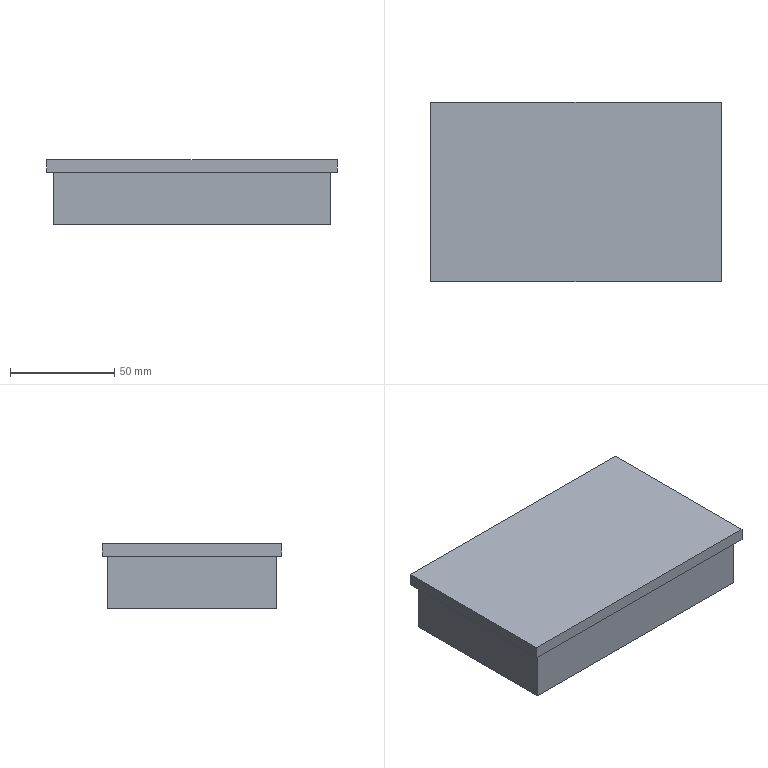Part | STEP file | Touch screen | 1 solid | 11 faces | box 139 x 86 x 31 mm | volume 341049 mm3 | plane 11
STEP:
#1=CARTESIAN_POINT('',(-66.5,40.5,0.));
#2=VERTEX_POINT('',#1);
#3=CARTESIAN_POINT('',(-66.5,-40.5,0.));
#4=VERTEX_POINT('',#3);
#5=CARTESIAN_POINT('',(-66.5,-40.5,0.));
#6=DIRECTION('',(0.,-1.,0.));
#7=VECTOR('',#6,1000.);
#8=LINE('',#5,#7);
#9=EDGE_CURVE('',#2,#4,#8,.T.);
#10=ORIENTED_EDGE('',*,*,#9,.T.);
#11=CARTESIAN_POINT('',(-66.5,-40.5,25.));
#12=VERTEX_POINT('',#11);
#13=CARTESIAN_POINT('',(-66.5,-40.5,25.));
#14=DIRECTION('',(0.,0.,-1.));
#15=VECTOR('',#14,1000.);
#16=LINE('',#13,#15);
#17=EDGE_CURVE('',#12,#4,#16,.T.);
#18=ORIENTED_EDGE('',*,*,#17,.F.);
#19=CARTESIAN_POINT('',(-66.5,40.5,25.));
#20=VERTEX_POINT('',#19);
#21=CARTESIAN_POINT('',(-66.5,-40.5,25.));
#22=DIRECTION('',(0.,-1.,0.));
#23=VECTOR('',#22,1000.);
#24=LINE('',#21,#23);
#25=EDGE_CURVE('',#20,#12,#24,.T.);
#26=ORIENTED_EDGE('',*,*,#25,.F.);
#27=CARTESIAN_POINT('',(-66.5,40.5,25.));
#28=DIRECTION('',(0.,0.,-1.));
#29=VECTOR('',#28,1000.);
#30=LINE('',#27,#29);
#31=EDGE_CURVE('',#20,#2,#30,.T.);
#32=ORIENTED_EDGE('',*,*,#31,.T.);
#33=EDGE_LOOP('',(#10,#18,#26,#32));
#34=FACE_OUTER_BOUND('',#33,.T.);
#35=CARTESIAN_POINT('',(-66.5,-40.5,25.));
#36=DIRECTION('',(1.,0.,0.));
#37=DIRECTION('',(0.,0.,-1.));
#38=AXIS2_PLACEMENT_3D('',#35,#36,#37);
#39=PLANE('',#38);
#40=ADVANCED_FACE('',(#34),#39,.F.);
#41=CARTESIAN_POINT('',(66.5,-40.5,0.));
#42=VERTEX_POINT('',#41);
#43=CARTESIAN_POINT('',(66.5,-40.5,0.));
#44=DIRECTION('',(1.,0.,0.));
#45=VECTOR('',#44,1000.);
#46=LINE('',#43,#45);
#47=EDGE_CURVE('',#4,#42,#46,.T.);
#48=ORIENTED_EDGE('',*,*,#47,.T.);
#49=CARTESIAN_POINT('',(66.5,-40.5,25.));
#50=VERTEX_POINT('',#49);
#51=CARTESIAN_POINT('',(66.5,-40.5,25.));
#52=DIRECTION('',(0.,0.,-1.));
#53=VECTOR('',#52,1000.);
#54=LINE('',#51,#53);
#55=EDGE_CURVE('',#50,#42,#54,.T.);
#56=ORIENTED_EDGE('',*,*,#55,.F.);
#57=CARTESIAN_POINT('',(66.5,-40.5,25.));
#58=DIRECTION('',(1.,0.,0.));
#59=VECTOR('',#58,1000.);
#60=LINE('',#57,#59);
#61=EDGE_CURVE('',#12,#50,#60,.T.);
#62=ORIENTED_EDGE('',*,*,#61,.F.);
#63=ORIENTED_EDGE('',*,*,#17,.T.);
#64=EDGE_LOOP('',(#48,#56,#62,#63));
#65=FACE_OUTER_BOUND('',#64,.T.);
#66=CARTESIAN_POINT('',(66.5,-40.5,25.));
#67=DIRECTION('',(0.,1.,0.));
#68=DIRECTION('',(0.,0.,1.));
#69=AXIS2_PLACEMENT_3D('',#66,#67,#68);
#70=PLANE('',#69);
#71=ADVANCED_FACE('',(#65),#70,.F.);
#72=CARTESIAN_POINT('',(66.5,40.5,0.));
#73=VERTEX_POINT('',#72);
#74=CARTESIAN_POINT('',(66.5,-40.5,0.));
#75=DIRECTION('',(0.,1.,0.));
#76=VECTOR('',#75,1000.);
#77=LINE('',#74,#76);
#78=EDGE_CURVE('',#42,#73,#77,.T.);
#79=ORIENTED_EDGE('',*,*,#78,.T.);
#80=CARTESIAN_POINT('',(66.5,40.5,25.));
#81=VERTEX_POINT('',#80);
#82=CARTESIAN_POINT('',(66.5,40.5,25.));
#83=DIRECTION('',(0.,0.,-1.));
#84=VECTOR('',#83,1000.);
#85=LINE('',#82,#84);
#86=EDGE_CURVE('',#81,#73,#85,.T.);
#87=ORIENTED_EDGE('',*,*,#86,.F.);
#88=CARTESIAN_POINT('',(66.5,-40.5,25.));
#89=DIRECTION('',(0.,1.,0.));
#90=VECTOR('',#89,1000.);
#91=LINE('',#88,#90);
#92=EDGE_CURVE('',#50,#81,#91,.T.);
#93=ORIENTED_EDGE('',*,*,#92,.F.);
#94=ORIENTED_EDGE('',*,*,#55,.T.);
#95=EDGE_LOOP('',(#79,#87,#93,#94));
#96=FACE_OUTER_BOUND('',#95,.T.);
#97=CARTESIAN_POINT('',(66.5,-40.5,25.));
#98=DIRECTION('',(-1.,0.,0.));
#99=DIRECTION('',(0.,0.,1.));
#100=AXIS2_PLACEMENT_3D('',#97,#98,#99);
#101=PLANE('',#100);
#102=ADVANCED_FACE('',(#96),#101,.F.);
#103=CARTESIAN_POINT('',(66.5,40.5,0.));
#104=DIRECTION('',(-1.,0.,0.));
#105=VECTOR('',#104,1000.);
#106=LINE('',#103,#105);
#107=EDGE_CURVE('',#73,#2,#106,.T.);
#108=ORIENTED_EDGE('',*,*,#107,.T.);
#109=ORIENTED_EDGE('',*,*,#31,.F.);
#110=CARTESIAN_POINT('',(66.5,40.5,25.));
#111=DIRECTION('',(-1.,0.,0.));
#112=VECTOR('',#111,1000.);
#113=LINE('',#110,#112);
#114=EDGE_CURVE('',#81,#20,#113,.T.);
#115=ORIENTED_EDGE('',*,*,#114,.F.);
#116=ORIENTED_EDGE('',*,*,#86,.T.);
#117=EDGE_LOOP('',(#108,#109,#115,#116));
#118=FACE_OUTER_BOUND('',#117,.T.);
#119=CARTESIAN_POINT('',(66.5,40.5,25.));
#120=DIRECTION('',(0.,-1.,0.));
#121=DIRECTION('',(0.,0.,-1.));
#122=AXIS2_PLACEMENT_3D('',#119,#120,#121);
#123=PLANE('',#122);
#124=ADVANCED_FACE('',(#118),#123,.F.);
#125=ORIENTED_EDGE('',*,*,#9,.F.);
#126=ORIENTED_EDGE('',*,*,#107,.F.);
#127=ORIENTED_EDGE('',*,*,#78,.F.);
#128=ORIENTED_EDGE('',*,*,#47,.F.);
#129=EDGE_LOOP('',(#125,#126,#127,#128));
#130=FACE_OUTER_BOUND('',#129,.T.);
#131=CARTESIAN_POINT('',(0.,0.,0.));
#132=DIRECTION('',(0.,0.,1.));
#133=DIRECTION('',(1.,0.,0.));
#134=AXIS2_PLACEMENT_3D('',#131,#132,#133);
#135=PLANE('',#134);
#136=ADVANCED_FACE('',(#130),#135,.F.);
#137=CARTESIAN_POINT('',(-69.5,43.,25.));
#138=VERTEX_POINT('',#137);
#139=CARTESIAN_POINT('',(-69.5,-43.,25.));
#140=VERTEX_POINT('',#139);
#141=CARTESIAN_POINT('',(-69.5,-43.,25.));
#142=DIRECTION('',(0.,-1.,0.));
#143=VECTOR('',#142,1000.);
#144=LINE('',#141,#143);
#145=EDGE_CURVE('',#138,#140,#144,.T.);
#146=ORIENTED_EDGE('',*,*,#145,.F.);
#147=CARTESIAN_POINT('',(69.5,43.,25.));
#148=VERTEX_POINT('',#147);
#149=CARTESIAN_POINT('',(69.5,43.,25.));
#150=DIRECTION('',(-1.,0.,0.));
#151=VECTOR('',#150,1000.);
#152=LINE('',#149,#151);
#153=EDGE_CURVE('',#148,#138,#152,.T.);
#154=ORIENTED_EDGE('',*,*,#153,.F.);
#155=CARTESIAN_POINT('',(69.5,-43.,25.));
#156=VERTEX_POINT('',#155);
#157=CARTESIAN_POINT('',(69.5,-43.,25.));
#158=DIRECTION('',(0.,1.,0.));
#159=VECTOR('',#158,1000.);
#160=LINE('',#157,#159);
#161=EDGE_CURVE('',#156,#148,#160,.T.);
#162=ORIENTED_EDGE('',*,*,#161,.F.);
#163=CARTESIAN_POINT('',(69.5,-43.,25.));
#164=DIRECTION('',(1.,0.,0.));
#165=VECTOR('',#164,1000.);
#166=LINE('',#163,#165);
#167=EDGE_CURVE('',#140,#156,#166,.T.);
#168=ORIENTED_EDGE('',*,*,#167,.F.);
#169=EDGE_LOOP('',(#146,#154,#162,#168));
#170=FACE_OUTER_BOUND('',#169,.T.);
#171=ORIENTED_EDGE('',*,*,#114,.T.);
#172=ORIENTED_EDGE('',*,*,#25,.T.);
#173=ORIENTED_EDGE('',*,*,#61,.T.);
#174=ORIENTED_EDGE('',*,*,#92,.T.);
#175=EDGE_LOOP('',(#171,#172,#173,#174));
#176=FACE_BOUND('',#175,.T.);
#177=CARTESIAN_POINT('',(0.,0.,25.));
#178=DIRECTION('',(0.,0.,1.));
#179=DIRECTION('',(1.,0.,0.));
#180=AXIS2_PLACEMENT_3D('',#177,#178,#179);
#181=PLANE('',#180);
#182=ADVANCED_FACE('',(#170,#176),#181,.F.);
#183=ORIENTED_EDGE('',*,*,#145,.T.);
#184=CARTESIAN_POINT('',(-69.5,-43.,31.));
#185=VERTEX_POINT('',#184);
#186=CARTESIAN_POINT('',(-69.5,-43.,31.));
#187=DIRECTION('',(0.,0.,-1.));
#188=VECTOR('',#187,1000.);
#189=LINE('',#186,#188);
#190=EDGE_CURVE('',#185,#140,#189,.T.);
#191=ORIENTED_EDGE('',*,*,#190,.F.);
#192=CARTESIAN_POINT('',(-69.5,43.,31.));
#193=VERTEX_POINT('',#192);
#194=CARTESIAN_POINT('',(-69.5,-43.,31.));
#195=DIRECTION('',(0.,-1.,0.));
#196=VECTOR('',#195,1000.);
#197=LINE('',#194,#196);
#198=EDGE_CURVE('',#193,#185,#197,.T.);
#199=ORIENTED_EDGE('',*,*,#198,.F.);
#200=CARTESIAN_POINT('',(-69.5,43.,31.));
#201=DIRECTION('',(0.,0.,-1.));
#202=VECTOR('',#201,1000.);
#203=LINE('',#200,#202);
#204=EDGE_CURVE('',#193,#138,#203,.T.);
#205=ORIENTED_EDGE('',*,*,#204,.T.);
#206=EDGE_LOOP('',(#183,#191,#199,#205));
#207=FACE_OUTER_BOUND('',#206,.T.);
#208=CARTESIAN_POINT('',(-69.5,-43.,31.));
#209=DIRECTION('',(1.,0.,0.));
#210=DIRECTION('',(0.,1.,0.));
#211=AXIS2_PLACEMENT_3D('',#208,#209,#210);
#212=PLANE('',#211);
#213=ADVANCED_FACE('',(#207),#212,.F.);
#214=ORIENTED_EDGE('',*,*,#167,.T.);
#215=CARTESIAN_POINT('',(69.5,-43.,31.));
#216=VERTEX_POINT('',#215);
#217=CARTESIAN_POINT('',(69.5,-43.,31.));
#218=DIRECTION('',(0.,0.,-1.));
#219=VECTOR('',#218,1000.);
#220=LINE('',#217,#219);
#221=EDGE_CURVE('',#216,#156,#220,.T.);
#222=ORIENTED_EDGE('',*,*,#221,.F.);
#223=CARTESIAN_POINT('',(69.5,-43.,31.));
#224=DIRECTION('',(1.,0.,0.));
#225=VECTOR('',#224,1000.);
#226=LINE('',#223,#225);
#227=EDGE_CURVE('',#185,#216,#226,.T.);
#228=ORIENTED_EDGE('',*,*,#227,.F.);
#229=ORIENTED_EDGE('',*,*,#190,.T.);
#230=EDGE_LOOP('',(#214,#222,#228,#229));
#231=FACE_OUTER_BOUND('',#230,.T.);
#232=CARTESIAN_POINT('',(69.5,-43.,31.));
#233=DIRECTION('',(0.,1.,0.));
#234=DIRECTION('',(0.,0.,1.));
#235=AXIS2_PLACEMENT_3D('',#232,#233,#234);
#236=PLANE('',#235);
#237=ADVANCED_FACE('',(#231),#236,.F.);
#238=ORIENTED_EDGE('',*,*,#161,.T.);
#239=CARTESIAN_POINT('',(69.5,43.,31.));
#240=VERTEX_POINT('',#239);
#241=CARTESIAN_POINT('',(69.5,43.,31.));
#242=DIRECTION('',(0.,0.,-1.));
#243=VECTOR('',#242,1000.);
#244=LINE('',#241,#243);
#245=EDGE_CURVE('',#240,#148,#244,.T.);
#246=ORIENTED_EDGE('',*,*,#245,.F.);
#247=CARTESIAN_POINT('',(69.5,-43.,31.));
#248=DIRECTION('',(0.,1.,0.));
#249=VECTOR('',#248,1000.);
#250=LINE('',#247,#249);
#251=EDGE_CURVE('',#216,#240,#250,.T.);
#252=ORIENTED_EDGE('',*,*,#251,.F.);
#253=ORIENTED_EDGE('',*,*,#221,.T.);
#254=EDGE_LOOP('',(#238,#246,#252,#253));
#255=FACE_OUTER_BOUND('',#254,.T.);
#256=CARTESIAN_POINT('',(69.5,-43.,31.));
#257=DIRECTION('',(-1.,0.,0.));
#258=DIRECTION('',(0.,0.,1.));
#259=AXIS2_PLACEMENT_3D('',#256,#257,#258);
#260=PLANE('',#259);
#261=ADVANCED_FACE('',(#255),#260,.F.);
#262=ORIENTED_EDGE('',*,*,#153,.T.);
#263=ORIENTED_EDGE('',*,*,#204,.F.);
#264=CARTESIAN_POINT('',(69.5,43.,31.));
#265=DIRECTION('',(-1.,0.,0.));
#266=VECTOR('',#265,1000.);
#267=LINE('',#264,#266);
#268=EDGE_CURVE('',#240,#193,#267,.T.);
#269=ORIENTED_EDGE('',*,*,#268,.F.);
#270=ORIENTED_EDGE('',*,*,#245,.T.);
#271=EDGE_LOOP('',(#262,#263,#269,#270));
#272=FACE_OUTER_BOUND('',#271,.T.);
#273=CARTESIAN_POINT('',(69.5,43.,31.));
#274=DIRECTION('',(0.,-1.,0.));
#275=DIRECTION('',(0.,0.,-1.));
#276=AXIS2_PLACEMENT_3D('',#273,#274,#275);
#277=PLANE('',#276);
#278=ADVANCED_FACE('',(#272),#277,.F.);
#279=ORIENTED_EDGE('',*,*,#198,.T.);
#280=ORIENTED_EDGE('',*,*,#227,.T.);
#281=ORIENTED_EDGE('',*,*,#251,.T.);
#282=ORIENTED_EDGE('',*,*,#268,.T.);
#283=EDGE_LOOP('',(#279,#280,#281,#282));
#284=FACE_OUTER_BOUND('',#283,.T.);
#285=CARTESIAN_POINT('',(0.,0.,31.));
#286=DIRECTION('',(0.,0.,1.));
#287=DIRECTION('',(1.,0.,0.));
#288=AXIS2_PLACEMENT_3D('',#285,#286,#287);
#289=PLANE('',#288);
#290=ADVANCED_FACE('',(#284),#289,.T.);
#291=CLOSED_SHELL('',(#40,#71,#102,#124,#136,#182,#213,#237,#261,#278,#290));
#292=MANIFOLD_SOLID_BREP('',#291);
#293=CARTESIAN_POINT('',(0.,0.,0.));
#294=DIRECTION('',(0.,0.,1.));
#295=DIRECTION('',(1.,0.,0.));
#296=AXIS2_PLACEMENT_3D('',#293,#294,#295);
#297=(LENGTH_UNIT()NAMED_UNIT(*)SI_UNIT(.MILLI.,.METRE.));
#298=UNCERTAINTY_MEASURE_WITH_UNIT(LENGTH_MEASURE(0.00001),#297,'','');
#299=(NAMED_UNIT(*)PLANE_ANGLE_UNIT()SI_UNIT($,.RADIAN.));
#300=(NAMED_UNIT(*)SI_UNIT($,.STERADIAN.)SOLID_ANGLE_UNIT());
#301=(GEOMETRIC_REPRESENTATION_CONTEXT(3)GLOBAL_UNCERTAINTY_ASSIGNED_CONTEXT((#298))GLOBAL_UNIT_ASSIGNED_CONTEXT((#297,#299,#300))REPRESENTATION_CONTEXT('',''));
#302=ADVANCED_BREP_SHAPE_REPRESENTATION('',(#292,#296),#301);